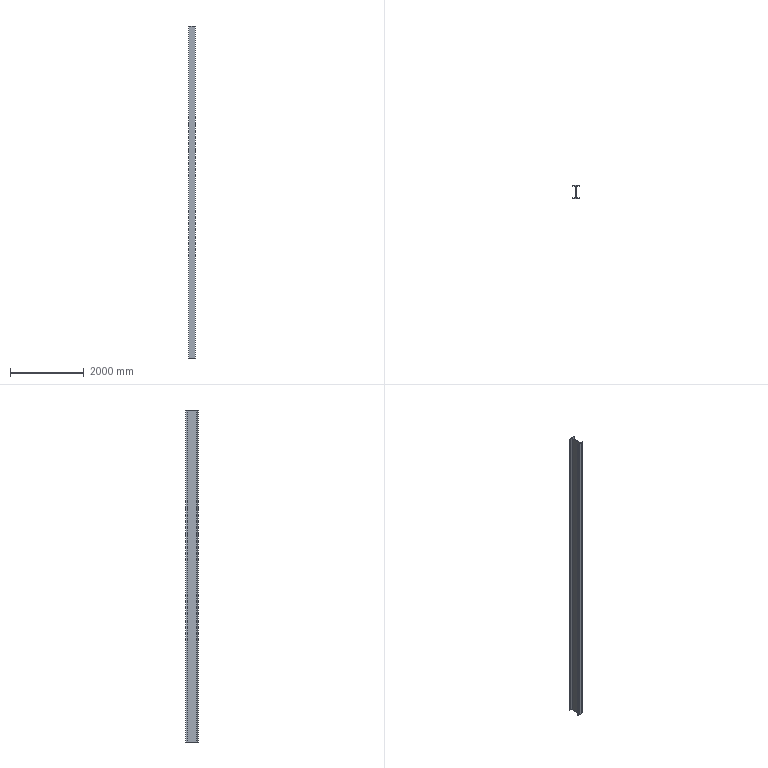Part | STEP file | 1 solid | 18 faces | box 175 x 350 x 9000 mm | volume 85369066 mm3 | plane 14 | cylinder 4 | commonest cylinder face diameters 80 x4
STEP:
#1=CARTESIAN_POINT('',(0.,0.,0.));
#2=DIRECTION('',(0.,0.,1.));
#3=DIRECTION('',(1.,0.,0.));
#4=AXIS2_PLACEMENT_3D('',#1,#2,#3);
#5=CARTESIAN_POINT('',(2499.715,-4168.542,-4500.));
#6=VERTEX_POINT('',#5);
#7=CARTESIAN_POINT('',(2499.715,-4156.542,-4500.));
#8=VERTEX_POINT('',#7);
#9=CARTESIAN_POINT('',(2499.715,-4156.542,-4500.));
#10=DIRECTION('',(0.,1.,0.));
#11=VECTOR('',#10,1.);
#12=LINE('',#9,#11);
#13=CARTESIAN_POINT('',(2499.715,-4156.542,4500.));
#14=DIRECTION('',(-1.,0.,0.));
#15=DIRECTION('',(0.,0.,1.));
#16=AXIS2_PLACEMENT_3D('',#13,#14,#15);
#17=PLANE('',#16);
#18=CARTESIAN_POINT('',(-9000.,0.));
#19=DIRECTION('',(0.,1.));
#20=VECTOR('',#19,1.);
#21=LINE('',#18,#20);
#22=(GEOMETRIC_REPRESENTATION_CONTEXT(2)PARAMETRIC_REPRESENTATION_CONTEXT()REPRESENTATION_CONTEXT('',''));
#23=DEFINITIONAL_REPRESENTATION('',(#21),#22);
#24=PCURVE('',#17,#23);
#25=CARTESIAN_POINT('',(2458.215,-4208.542,-4500.));
#26=DIRECTION('',(0.,0.,1.));
#27=DIRECTION('',(1.,0.,0.));
#28=AXIS2_PLACEMENT_3D('',#25,#26,#27);
#29=PLANE('',#28);
#30=CARTESIAN_POINT('',(41.5,52.));
#31=DIRECTION('',(0.,1.));
#32=VECTOR('',#31,1.);
#33=LINE('',#30,#32);
#34=(GEOMETRIC_REPRESENTATION_CONTEXT(2)PARAMETRIC_REPRESENTATION_CONTEXT()REPRESENTATION_CONTEXT('',''));
#35=DEFINITIONAL_REPRESENTATION('',(#33),#34);
#36=PCURVE('',#29,#35);
#37=SURFACE_CURVE('',#12,(#24,#36),.PCURVE_S1.);
#38=EDGE_CURVE('',#6,#8,#37,.T.);
#39=ORIENTED_EDGE('',*,*,#38,.T.);
#40=CARTESIAN_POINT('',(2499.715,-4156.542,4500.));
#41=VERTEX_POINT('',#40);
#42=CARTESIAN_POINT('',(2499.715,-4156.542,4500.));
#43=DIRECTION('',(0.,0.,-1.));
#44=VECTOR('',#43,1.);
#45=LINE('',#42,#44);
#46=CARTESIAN_POINT('',(0.,0.));
#47=DIRECTION('',(-1.,0.));
#48=VECTOR('',#47,1.);
#49=LINE('',#46,#48);
#50=(GEOMETRIC_REPRESENTATION_CONTEXT(2)PARAMETRIC_REPRESENTATION_CONTEXT()REPRESENTATION_CONTEXT('',''));
#51=DEFINITIONAL_REPRESENTATION('',(#49),#50);
#52=PCURVE('',#17,#51);
#53=CARTESIAN_POINT('',(2499.715,-4156.542,4500.));
#54=DIRECTION('',(0.,-1.,0.));
#55=DIRECTION('',(0.,0.,-1.));
#56=AXIS2_PLACEMENT_3D('',#53,#54,#55);
#57=PLANE('',#56);
#58=CARTESIAN_POINT('',(0.,0.));
#59=DIRECTION('',(1.,0.));
#60=VECTOR('',#59,1.);
#61=LINE('',#58,#60);
#62=(GEOMETRIC_REPRESENTATION_CONTEXT(2)PARAMETRIC_REPRESENTATION_CONTEXT()REPRESENTATION_CONTEXT('',''));
#63=DEFINITIONAL_REPRESENTATION('',(#61),#62);
#64=PCURVE('',#57,#63);
#65=SURFACE_CURVE('',#45,(#52,#64),.PCURVE_S1.);
#66=EDGE_CURVE('',#41,#8,#65,.T.);
#67=ORIENTED_EDGE('',*,*,#66,.F.);
#68=CARTESIAN_POINT('',(2499.715,-4168.542,4500.));
#69=VERTEX_POINT('',#68);
#70=CARTESIAN_POINT('',(2499.715,-4156.542,4500.));
#71=DIRECTION('',(0.,1.,0.));
#72=VECTOR('',#71,1.);
#73=LINE('',#70,#72);
#74=CARTESIAN_POINT('',(0.,0.));
#75=DIRECTION('',(0.,1.));
#76=VECTOR('',#75,1.);
#77=LINE('',#74,#76);
#78=(GEOMETRIC_REPRESENTATION_CONTEXT(2)PARAMETRIC_REPRESENTATION_CONTEXT()REPRESENTATION_CONTEXT('',''));
#79=DEFINITIONAL_REPRESENTATION('',(#77),#78);
#80=PCURVE('',#17,#79);
#81=CARTESIAN_POINT('',(2458.215,-4208.542,4500.));
#82=DIRECTION('',(0.,0.,1.));
#83=DIRECTION('',(1.,0.,0.));
#84=AXIS2_PLACEMENT_3D('',#81,#82,#83);
#85=PLANE('',#84);
#86=CARTESIAN_POINT('',(41.5,52.));
#87=DIRECTION('',(0.,1.));
#88=VECTOR('',#87,1.);
#89=LINE('',#86,#88);
#90=(GEOMETRIC_REPRESENTATION_CONTEXT(2)PARAMETRIC_REPRESENTATION_CONTEXT()REPRESENTATION_CONTEXT('',''));
#91=DEFINITIONAL_REPRESENTATION('',(#89),#90);
#92=PCURVE('',#85,#91);
#93=SURFACE_CURVE('',#73,(#80,#92),.PCURVE_S1.);
#94=EDGE_CURVE('',#69,#41,#93,.T.);
#95=ORIENTED_EDGE('',*,*,#94,.F.);
#96=CARTESIAN_POINT('',(2499.715,-4168.542,4500.));
#97=DIRECTION('',(0.,0.,-1.));
#98=VECTOR('',#97,1.);
#99=LINE('',#96,#98);
#100=CARTESIAN_POINT('',(0.,-12.));
#101=DIRECTION('',(-1.,0.));
#102=VECTOR('',#101,1.);
#103=LINE('',#100,#102);
#104=(GEOMETRIC_REPRESENTATION_CONTEXT(2)PARAMETRIC_REPRESENTATION_CONTEXT()REPRESENTATION_CONTEXT('',''));
#105=DEFINITIONAL_REPRESENTATION('',(#103),#104);
#106=PCURVE('',#17,#105);
#107=CARTESIAN_POINT('',(2499.715,-4168.542,4500.));
#108=DIRECTION('',(0.,1.,0.));
#109=DIRECTION('',(0.,0.,1.));
#110=AXIS2_PLACEMENT_3D('',#107,#108,#109);
#111=PLANE('',#110);
#112=CARTESIAN_POINT('',(0.,0.));
#113=DIRECTION('',(-1.,0.));
#114=VECTOR('',#113,1.);
#115=LINE('',#112,#114);
#116=(GEOMETRIC_REPRESENTATION_CONTEXT(2)PARAMETRIC_REPRESENTATION_CONTEXT()REPRESENTATION_CONTEXT('',''));
#117=DEFINITIONAL_REPRESENTATION('',(#115),#116);
#118=PCURVE('',#111,#117);
#119=SURFACE_CURVE('',#99,(#106,#118),.PCURVE_S1.);
#120=EDGE_CURVE('',#69,#6,#119,.T.);
#121=ORIENTED_EDGE('',*,*,#120,.T.);
#122=EDGE_LOOP('',(#39,#67,#95,#121));
#123=FACE_BOUND('',#122,.T.);
#124=ADVANCED_FACE('',(#123),#17,.F.);
#125=CARTESIAN_POINT('',(2324.715,-4156.542,-4500.));
#126=VERTEX_POINT('',#125);
#127=CARTESIAN_POINT('',(2499.715,-4156.542,-4500.));
#128=DIRECTION('',(-1.,0.,0.));
#129=VECTOR('',#128,1.);
#130=LINE('',#127,#129);
#131=CARTESIAN_POINT('',(9000.,0.));
#132=DIRECTION('',(0.,-1.));
#133=VECTOR('',#132,1.);
#134=LINE('',#131,#133);
#135=(GEOMETRIC_REPRESENTATION_CONTEXT(2)PARAMETRIC_REPRESENTATION_CONTEXT()REPRESENTATION_CONTEXT('',''));
#136=DEFINITIONAL_REPRESENTATION('',(#134),#135);
#137=PCURVE('',#57,#136);
#138=CARTESIAN_POINT('',(41.5,52.));
#139=DIRECTION('',(-1.,0.));
#140=VECTOR('',#139,1.);
#141=LINE('',#138,#140);
#142=(GEOMETRIC_REPRESENTATION_CONTEXT(2)PARAMETRIC_REPRESENTATION_CONTEXT()REPRESENTATION_CONTEXT('',''));
#143=DEFINITIONAL_REPRESENTATION('',(#141),#142);
#144=PCURVE('',#29,#143);
#145=SURFACE_CURVE('',#130,(#137,#144),.PCURVE_S1.);
#146=EDGE_CURVE('',#8,#126,#145,.T.);
#147=ORIENTED_EDGE('',*,*,#146,.T.);
#148=CARTESIAN_POINT('',(2324.715,-4156.542,4500.));
#149=VERTEX_POINT('',#148);
#150=CARTESIAN_POINT('',(2324.715,-4156.542,4500.));
#151=DIRECTION('',(0.,0.,-1.));
#152=VECTOR('',#151,1.);
#153=LINE('',#150,#152);
#154=CARTESIAN_POINT('',(0.,-175.));
#155=DIRECTION('',(1.,0.));
#156=VECTOR('',#155,1.);
#157=LINE('',#154,#156);
#158=(GEOMETRIC_REPRESENTATION_CONTEXT(2)PARAMETRIC_REPRESENTATION_CONTEXT()REPRESENTATION_CONTEXT('',''));
#159=DEFINITIONAL_REPRESENTATION('',(#157),#158);
#160=PCURVE('',#57,#159);
#161=CARTESIAN_POINT('',(2324.715,-4156.542,4500.));
#162=DIRECTION('',(1.,0.,0.));
#163=DIRECTION('',(0.,0.,-1.));
#164=AXIS2_PLACEMENT_3D('',#161,#162,#163);
#165=PLANE('',#164);
#166=CARTESIAN_POINT('',(0.,0.));
#167=DIRECTION('',(1.,0.));
#168=VECTOR('',#167,1.);
#169=LINE('',#166,#168);
#170=(GEOMETRIC_REPRESENTATION_CONTEXT(2)PARAMETRIC_REPRESENTATION_CONTEXT()REPRESENTATION_CONTEXT('',''));
#171=DEFINITIONAL_REPRESENTATION('',(#169),#170);
#172=PCURVE('',#165,#171);
#173=SURFACE_CURVE('',#153,(#160,#172),.PCURVE_S1.);
#174=EDGE_CURVE('',#149,#126,#173,.T.);
#175=ORIENTED_EDGE('',*,*,#174,.F.);
#176=CARTESIAN_POINT('',(2499.715,-4156.542,4500.));
#177=DIRECTION('',(-1.,0.,0.));
#178=VECTOR('',#177,1.);
#179=LINE('',#176,#178);
#180=CARTESIAN_POINT('',(0.,0.));
#181=DIRECTION('',(0.,-1.));
#182=VECTOR('',#181,1.);
#183=LINE('',#180,#182);
#184=(GEOMETRIC_REPRESENTATION_CONTEXT(2)PARAMETRIC_REPRESENTATION_CONTEXT()REPRESENTATION_CONTEXT('',''));
#185=DEFINITIONAL_REPRESENTATION('',(#183),#184);
#186=PCURVE('',#57,#185);
#187=CARTESIAN_POINT('',(41.5,52.));
#188=DIRECTION('',(-1.,0.));
#189=VECTOR('',#188,1.);
#190=LINE('',#187,#189);
#191=(GEOMETRIC_REPRESENTATION_CONTEXT(2)PARAMETRIC_REPRESENTATION_CONTEXT()REPRESENTATION_CONTEXT('',''));
#192=DEFINITIONAL_REPRESENTATION('',(#190),#191);
#193=PCURVE('',#85,#192);
#194=SURFACE_CURVE('',#179,(#186,#193),.PCURVE_S1.);
#195=EDGE_CURVE('',#41,#149,#194,.T.);
#196=ORIENTED_EDGE('',*,*,#195,.F.);
#197=ORIENTED_EDGE('',*,*,#66,.T.);
#198=EDGE_LOOP('',(#147,#175,#196,#197));
#199=FACE_BOUND('',#198,.T.);
#200=ADVANCED_FACE('',(#199),#57,.F.);
#201=CARTESIAN_POINT('',(2324.715,-4168.542,-4500.));
#202=VERTEX_POINT('',#201);
#203=CARTESIAN_POINT('',(2324.715,-4156.542,-4500.));
#204=DIRECTION('',(0.,-1.,0.));
#205=VECTOR('',#204,1.);
#206=LINE('',#203,#205);
#207=CARTESIAN_POINT('',(9000.,0.));
#208=DIRECTION('',(0.,-1.));
#209=VECTOR('',#208,1.);
#210=LINE('',#207,#209);
#211=(GEOMETRIC_REPRESENTATION_CONTEXT(2)PARAMETRIC_REPRESENTATION_CONTEXT()REPRESENTATION_CONTEXT('',''));
#212=DEFINITIONAL_REPRESENTATION('',(#210),#211);
#213=PCURVE('',#165,#212);
#214=CARTESIAN_POINT('',(-133.5,52.));
#215=DIRECTION('',(0.,-1.));
#216=VECTOR('',#215,1.);
#217=LINE('',#214,#216);
#218=(GEOMETRIC_REPRESENTATION_CONTEXT(2)PARAMETRIC_REPRESENTATION_CONTEXT()REPRESENTATION_CONTEXT('',''));
#219=DEFINITIONAL_REPRESENTATION('',(#217),#218);
#220=PCURVE('',#29,#219);
#221=SURFACE_CURVE('',#206,(#213,#220),.PCURVE_S1.);
#222=EDGE_CURVE('',#126,#202,#221,.T.);
#223=ORIENTED_EDGE('',*,*,#222,.T.);
#224=CARTESIAN_POINT('',(2324.715,-4168.542,4500.));
#225=VERTEX_POINT('',#224);
#226=CARTESIAN_POINT('',(2324.715,-4168.542,4500.));
#227=DIRECTION('',(0.,0.,-1.));
#228=VECTOR('',#227,1.);
#229=LINE('',#226,#228);
#230=CARTESIAN_POINT('',(0.,-12.));
#231=DIRECTION('',(1.,0.));
#232=VECTOR('',#231,1.);
#233=LINE('',#230,#232);
#234=(GEOMETRIC_REPRESENTATION_CONTEXT(2)PARAMETRIC_REPRESENTATION_CONTEXT()REPRESENTATION_CONTEXT('',''));
#235=DEFINITIONAL_REPRESENTATION('',(#233),#234);
#236=PCURVE('',#165,#235);
#237=CARTESIAN_POINT('',(2366.215,-4168.542,4500.));
#238=DIRECTION('',(0.,1.,0.));
#239=DIRECTION('',(0.,0.,1.));
#240=AXIS2_PLACEMENT_3D('',#237,#238,#239);
#241=PLANE('',#240);
#242=CARTESIAN_POINT('',(0.,-41.5));
#243=DIRECTION('',(-1.,0.));
#244=VECTOR('',#243,1.);
#245=LINE('',#242,#244);
#246=(GEOMETRIC_REPRESENTATION_CONTEXT(2)PARAMETRIC_REPRESENTATION_CONTEXT()REPRESENTATION_CONTEXT('',''));
#247=DEFINITIONAL_REPRESENTATION('',(#245),#246);
#248=PCURVE('',#241,#247);
#249=SURFACE_CURVE('',#229,(#236,#248),.PCURVE_S1.);
#250=EDGE_CURVE('',#225,#202,#249,.T.);
#251=ORIENTED_EDGE('',*,*,#250,.F.);
#252=CARTESIAN_POINT('',(2324.715,-4156.542,4500.));
#253=DIRECTION('',(0.,-1.,0.));
#254=VECTOR('',#253,1.);
#255=LINE('',#252,#254);
#256=CARTESIAN_POINT('',(0.,0.));
#257=DIRECTION('',(0.,-1.));
#258=VECTOR('',#257,1.);
#259=LINE('',#256,#258);
#260=(GEOMETRIC_REPRESENTATION_CONTEXT(2)PARAMETRIC_REPRESENTATION_CONTEXT()REPRESENTATION_CONTEXT('',''));
#261=DEFINITIONAL_REPRESENTATION('',(#259),#260);
#262=PCURVE('',#165,#261);
#263=CARTESIAN_POINT('',(-133.5,52.));
#264=DIRECTION('',(0.,-1.));
#265=VECTOR('',#264,1.);
#266=LINE('',#263,#265);
#267=(GEOMETRIC_REPRESENTATION_CONTEXT(2)PARAMETRIC_REPRESENTATION_CONTEXT()REPRESENTATION_CONTEXT('',''));
#268=DEFINITIONAL_REPRESENTATION('',(#266),#267);
#269=PCURVE('',#85,#268);
#270=SURFACE_CURVE('',#255,(#262,#269),.PCURVE_S1.);
#271=EDGE_CURVE('',#149,#225,#270,.T.);
#272=ORIENTED_EDGE('',*,*,#271,.F.);
#273=ORIENTED_EDGE('',*,*,#174,.T.);
#274=EDGE_LOOP('',(#223,#251,#272,#273));
#275=FACE_BOUND('',#274,.T.);
#276=ADVANCED_FACE('',(#275),#165,.F.);
#277=CARTESIAN_POINT('',(2366.215,-4168.542,-4500.));
#278=VERTEX_POINT('',#277);
#279=CARTESIAN_POINT('',(2366.215,-4168.542,-4500.));
#280=DIRECTION('',(1.,0.,0.));
#281=VECTOR('',#280,1.);
#282=LINE('',#279,#281);
#283=CARTESIAN_POINT('',(-9000.,0.));
#284=DIRECTION('',(0.,1.));
#285=VECTOR('',#284,1.);
#286=LINE('',#283,#285);
#287=(GEOMETRIC_REPRESENTATION_CONTEXT(2)PARAMETRIC_REPRESENTATION_CONTEXT()REPRESENTATION_CONTEXT('',''));
#288=DEFINITIONAL_REPRESENTATION('',(#286),#287);
#289=PCURVE('',#241,#288);
#290=CARTESIAN_POINT('',(-92.,40.));
#291=DIRECTION('',(1.,0.));
#292=VECTOR('',#291,1.);
#293=LINE('',#290,#292);
#294=(GEOMETRIC_REPRESENTATION_CONTEXT(2)PARAMETRIC_REPRESENTATION_CONTEXT()REPRESENTATION_CONTEXT('',''));
#295=DEFINITIONAL_REPRESENTATION('',(#293),#294);
#296=PCURVE('',#29,#295);
#297=SURFACE_CURVE('',#282,(#289,#296),.PCURVE_S1.);
#298=EDGE_CURVE('',#202,#278,#297,.T.);
#299=ORIENTED_EDGE('',*,*,#298,.T.);
#300=CARTESIAN_POINT('',(2366.215,-4168.542,4500.));
#301=VERTEX_POINT('',#300);
#302=CARTESIAN_POINT('',(2366.215,-4168.542,4500.));
#303=DIRECTION('',(0.,0.,-1.));
#304=VECTOR('',#303,1.);
#305=LINE('',#302,#304);
#306=CARTESIAN_POINT('',(0.,0.));
#307=DIRECTION('',(-1.,0.));
#308=VECTOR('',#307,1.);
#309=LINE('',#306,#308);
#310=(GEOMETRIC_REPRESENTATION_CONTEXT(2)PARAMETRIC_REPRESENTATION_CONTEXT()REPRESENTATION_CONTEXT('',''));
#311=DEFINITIONAL_REPRESENTATION('',(#309),#310);
#312=PCURVE('',#241,#311);
#313=CARTESIAN_POINT('',(2366.215,-4208.542,4500.));
#314=DIRECTION('',(0.,0.,-1.));
#315=DIRECTION('',(-1.,0.,0.));
#316=AXIS2_PLACEMENT_3D('',#313,#314,#315);
#317=CYLINDRICAL_SURFACE('',#316,40.);
#318=CARTESIAN_POINT('',(1.571,0.));
#319=DIRECTION('',(0.,1.));
#320=VECTOR('',#319,1.);
#321=LINE('',#318,#320);
#322=(GEOMETRIC_REPRESENTATION_CONTEXT(2)PARAMETRIC_REPRESENTATION_CONTEXT()REPRESENTATION_CONTEXT('',''));
#323=DEFINITIONAL_REPRESENTATION('',(#321),#322);
#324=PCURVE('',#317,#323);
#325=SURFACE_CURVE('',#305,(#312,#324),.PCURVE_S1.);
#326=EDGE_CURVE('',#301,#278,#325,.T.);
#327=ORIENTED_EDGE('',*,*,#326,.F.);
#328=CARTESIAN_POINT('',(2366.215,-4168.542,4500.));
#329=DIRECTION('',(1.,0.,0.));
#330=VECTOR('',#329,1.);
#331=LINE('',#328,#330);
#332=CARTESIAN_POINT('',(0.,0.));
#333=DIRECTION('',(0.,1.));
#334=VECTOR('',#333,1.);
#335=LINE('',#332,#334);
#336=(GEOMETRIC_REPRESENTATION_CONTEXT(2)PARAMETRIC_REPRESENTATION_CONTEXT()REPRESENTATION_CONTEXT('',''));
#337=DEFINITIONAL_REPRESENTATION('',(#335),#336);
#338=PCURVE('',#241,#337);
#339=CARTESIAN_POINT('',(-92.,40.));
#340=DIRECTION('',(1.,0.));
#341=VECTOR('',#340,1.);
#342=LINE('',#339,#341);
#343=(GEOMETRIC_REPRESENTATION_CONTEXT(2)PARAMETRIC_REPRESENTATION_CONTEXT()REPRESENTATION_CONTEXT('',''));
#344=DEFINITIONAL_REPRESENTATION('',(#342),#343);
#345=PCURVE('',#85,#344);
#346=SURFACE_CURVE('',#331,(#338,#345),.PCURVE_S1.);
#347=EDGE_CURVE('',#225,#301,#346,.T.);
#348=ORIENTED_EDGE('',*,*,#347,.F.);
#349=ORIENTED_EDGE('',*,*,#250,.T.);
#350=EDGE_LOOP('',(#299,#327,#348,#349));
#351=FACE_BOUND('',#350,.T.);
#352=ADVANCED_FACE('',(#351),#241,.F.);
#353=ORIENTED_EDGE('',*,*,#326,.F.);
#354=CARTESIAN_POINT('',(2406.215,-4208.542,4500.));
#355=VERTEX_POINT('',#354);
#356=CARTESIAN_POINT('',(2366.215,-4208.542,4500.));
#357=DIRECTION('',(0.,0.,-1.));
#358=DIRECTION('',(1.,0.,0.));
#359=AXIS2_PLACEMENT_3D('',#356,#357,#358);
#360=CIRCLE('',#359,40.);
#361=CARTESIAN_POINT('',(-3.142,0.));
#362=DIRECTION('',(1.,0.));
#363=VECTOR('',#362,1.);
#364=LINE('',#361,#363);
#365=(GEOMETRIC_REPRESENTATION_CONTEXT(2)PARAMETRIC_REPRESENTATION_CONTEXT()REPRESENTATION_CONTEXT('',''));
#366=DEFINITIONAL_REPRESENTATION('',(#364),#365);
#367=PCURVE('',#317,#366);
#368=CARTESIAN_POINT('',(-52.,0.));
#369=CARTESIAN_POINT('',(-52.,-69.282));
#370=CARTESIAN_POINT('',(-112.,-34.641));
#371=CARTESIAN_POINT('',(-172.,0.));
#372=CARTESIAN_POINT('',(-112.,34.641));
#373=CARTESIAN_POINT('',(-52.,69.282));
#374=CARTESIAN_POINT('',(-52.,0.));
#375=(BOUNDED_CURVE()B_SPLINE_CURVE(2,(#368,#369,#370,#371,#372,#373,#374),.UNSPECIFIED.,.T.,.F.)B_SPLINE_CURVE_WITH_KNOTS((1,2,2,2,2,1),(-2.094,0.,2.094,4.189,6.283,8.378),.UNSPECIFIED.)CURVE()GEOMETRIC_REPRESENTATION_ITEM()RATIONAL_B_SPLINE_CURVE((1.,0.5,1.,0.5,1.,0.5,1.))REPRESENTATION_ITEM(''));
#376=(GEOMETRIC_REPRESENTATION_CONTEXT(2)PARAMETRIC_REPRESENTATION_CONTEXT()REPRESENTATION_CONTEXT('',''));
#377=DEFINITIONAL_REPRESENTATION('',(#375),#376);
#378=PCURVE('',#85,#377);
#379=SURFACE_CURVE('',#360,(#367,#378),.PCURVE_S1.);
#380=EDGE_CURVE('',#301,#355,#379,.T.);
#381=ORIENTED_EDGE('',*,*,#380,.T.);
#382=CARTESIAN_POINT('',(2406.215,-4208.542,-4500.));
#383=VERTEX_POINT('',#382);
#384=CARTESIAN_POINT('',(2406.215,-4208.542,4500.));
#385=DIRECTION('',(0.,0.,-1.));
#386=VECTOR('',#385,1.);
#387=LINE('',#384,#386);
#388=CARTESIAN_POINT('',(3.142,0.));
#389=DIRECTION('',(0.,1.));
#390=VECTOR('',#389,1.);
#391=LINE('',#388,#390);
#392=(GEOMETRIC_REPRESENTATION_CONTEXT(2)PARAMETRIC_REPRESENTATION_CONTEXT()REPRESENTATION_CONTEXT('',''));
#393=DEFINITIONAL_REPRESENTATION('',(#391),#392);
#394=PCURVE('',#317,#393);
#395=CARTESIAN_POINT('',(2406.215,-4208.542,4500.));
#396=DIRECTION('',(1.,0.,0.));
#397=DIRECTION('',(0.,0.,-1.));
#398=AXIS2_PLACEMENT_3D('',#395,#396,#397);
#399=PLANE('',#398);
#400=CARTESIAN_POINT('',(0.,0.));
#401=DIRECTION('',(1.,0.));
#402=VECTOR('',#401,1.);
#403=LINE('',#400,#402);
#404=(GEOMETRIC_REPRESENTATION_CONTEXT(2)PARAMETRIC_REPRESENTATION_CONTEXT()REPRESENTATION_CONTEXT('',''));
#405=DEFINITIONAL_REPRESENTATION('',(#403),#404);
#406=PCURVE('',#399,#405);
#407=SURFACE_CURVE('',#387,(#394,#406),.PCURVE_S1.);
#408=EDGE_CURVE('',#355,#383,#407,.T.);
#409=ORIENTED_EDGE('',*,*,#408,.T.);
#410=CARTESIAN_POINT('',(2366.215,-4208.542,-4500.));
#411=DIRECTION('',(0.,0.,-1.));
#412=DIRECTION('',(1.,0.,0.));
#413=AXIS2_PLACEMENT_3D('',#410,#411,#412);
#414=CIRCLE('',#413,40.);
#415=CARTESIAN_POINT('',(-3.142,9000.));
#416=DIRECTION('',(1.,0.));
#417=VECTOR('',#416,1.);
#418=LINE('',#415,#417);
#419=(GEOMETRIC_REPRESENTATION_CONTEXT(2)PARAMETRIC_REPRESENTATION_CONTEXT()REPRESENTATION_CONTEXT('',''));
#420=DEFINITIONAL_REPRESENTATION('',(#418),#419);
#421=PCURVE('',#317,#420);
#422=CARTESIAN_POINT('',(-52.,0.));
#423=CARTESIAN_POINT('',(-52.,-69.282));
#424=CARTESIAN_POINT('',(-112.,-34.641));
#425=CARTESIAN_POINT('',(-172.,0.));
#426=CARTESIAN_POINT('',(-112.,34.641));
#427=CARTESIAN_POINT('',(-52.,69.282));
#428=CARTESIAN_POINT('',(-52.,0.));
#429=(BOUNDED_CURVE()B_SPLINE_CURVE(2,(#422,#423,#424,#425,#426,#427,#428),.UNSPECIFIED.,.T.,.F.)B_SPLINE_CURVE_WITH_KNOTS((1,2,2,2,2,1),(-2.094,0.,2.094,4.189,6.283,8.378),.UNSPECIFIED.)CURVE()GEOMETRIC_REPRESENTATION_ITEM()RATIONAL_B_SPLINE_CURVE((1.,0.5,1.,0.5,1.,0.5,1.))REPRESENTATION_ITEM(''));
#430=(GEOMETRIC_REPRESENTATION_CONTEXT(2)PARAMETRIC_REPRESENTATION_CONTEXT()REPRESENTATION_CONTEXT('',''));
#431=DEFINITIONAL_REPRESENTATION('',(#429),#430);
#432=PCURVE('',#29,#431);
#433=SURFACE_CURVE('',#414,(#421,#432),.PCURVE_S1.);
#434=EDGE_CURVE('',#278,#383,#433,.T.);
#435=ORIENTED_EDGE('',*,*,#434,.F.);
#436=EDGE_LOOP('',(#353,#381,#409,#435));
#437=FACE_BOUND('',#436,.F.);
#438=ADVANCED_FACE('',(#437),#317,.F.);
#439=CARTESIAN_POINT('',(2406.215,-4454.542,-4500.));
#440=VERTEX_POINT('',#439);
#441=CARTESIAN_POINT('',(2406.215,-4208.542,-4500.));
#442=DIRECTION('',(0.,-1.,0.));
#443=VECTOR('',#442,1.);
#444=LINE('',#441,#443);
#445=CARTESIAN_POINT('',(9000.,0.));
#446=DIRECTION('',(0.,-1.));
#447=VECTOR('',#446,1.);
#448=LINE('',#445,#447);
#449=(GEOMETRIC_REPRESENTATION_CONTEXT(2)PARAMETRIC_REPRESENTATION_CONTEXT()REPRESENTATION_CONTEXT('',''));
#450=DEFINITIONAL_REPRESENTATION('',(#448),#449);
#451=PCURVE('',#399,#450);
#452=CARTESIAN_POINT('',(-52.,0.));
#453=DIRECTION('',(0.,-1.));
#454=VECTOR('',#453,1.);
#455=LINE('',#452,#454);
#456=(GEOMETRIC_REPRESENTATION_CONTEXT(2)PARAMETRIC_REPRESENTATION_CONTEXT()REPRESENTATION_CONTEXT('',''));
#457=DEFINITIONAL_REPRESENTATION('',(#455),#456);
#458=PCURVE('',#29,#457);
#459=SURFACE_CURVE('',#444,(#451,#458),.PCURVE_S1.);
#460=EDGE_CURVE('',#383,#440,#459,.T.);
#461=ORIENTED_EDGE('',*,*,#460,.T.);
#462=CARTESIAN_POINT('',(2406.215,-4454.542,4500.));
#463=VERTEX_POINT('',#462);
#464=CARTESIAN_POINT('',(2406.215,-4454.542,4500.));
#465=DIRECTION('',(0.,0.,-1.));
#466=VECTOR('',#465,1.);
#467=LINE('',#464,#466);
#468=CARTESIAN_POINT('',(0.,-246.));
#469=DIRECTION('',(1.,0.));
#470=VECTOR('',#469,1.);
#471=LINE('',#468,#470);
#472=(GEOMETRIC_REPRESENTATION_CONTEXT(2)PARAMETRIC_REPRESENTATION_CONTEXT()REPRESENTATION_CONTEXT('',''));
#473=DEFINITIONAL_REPRESENTATION('',(#471),#472);
#474=PCURVE('',#399,#473);
#475=CARTESIAN_POINT('',(2366.215,-4454.542,4500.));
#476=DIRECTION('',(0.,0.,-1.));
#477=DIRECTION('',(-1.,0.,0.));
#478=AXIS2_PLACEMENT_3D('',#475,#476,#477);
#479=CYLINDRICAL_SURFACE('',#478,40.);
#480=CARTESIAN_POINT('',(3.142,0.));
#481=DIRECTION('',(0.,1.));
#482=VECTOR('',#481,1.);
#483=LINE('',#480,#482);
#484=(GEOMETRIC_REPRESENTATION_CONTEXT(2)PARAMETRIC_REPRESENTATION_CONTEXT()REPRESENTATION_CONTEXT('',''));
#485=DEFINITIONAL_REPRESENTATION('',(#483),#484);
#486=PCURVE('',#479,#485);
#487=SURFACE_CURVE('',#467,(#474,#486),.PCURVE_S1.);
#488=EDGE_CURVE('',#463,#440,#487,.T.);
#489=ORIENTED_EDGE('',*,*,#488,.F.);
#490=CARTESIAN_POINT('',(2406.215,-4208.542,4500.));
#491=DIRECTION('',(0.,-1.,0.));
#492=VECTOR('',#491,1.);
#493=LINE('',#490,#492);
#494=CARTESIAN_POINT('',(0.,0.));
#495=DIRECTION('',(0.,-1.));
#496=VECTOR('',#495,1.);
#497=LINE('',#494,#496);
#498=(GEOMETRIC_REPRESENTATION_CONTEXT(2)PARAMETRIC_REPRESENTATION_CONTEXT()REPRESENTATION_CONTEXT('',''));
#499=DEFINITIONAL_REPRESENTATION('',(#497),#498);
#500=PCURVE('',#399,#499);
#501=CARTESIAN_POINT('',(-52.,0.));
#502=DIRECTION('',(0.,-1.));
#503=VECTOR('',#502,1.);
#504=LINE('',#501,#503);
#505=(GEOMETRIC_REPRESENTATION_CONTEXT(2)PARAMETRIC_REPRESENTATION_CONTEXT()REPRESENTATION_CONTEXT('',''));
#506=DEFINITIONAL_REPRESENTATION('',(#504),#505);
#507=PCURVE('',#85,#506);
#508=SURFACE_CURVE('',#493,(#500,#507),.PCURVE_S1.);
#509=EDGE_CURVE('',#355,#463,#508,.T.);
#510=ORIENTED_EDGE('',*,*,#509,.F.);
#511=ORIENTED_EDGE('',*,*,#408,.T.);
#512=EDGE_LOOP('',(#461,#489,#510,#511));
#513=FACE_BOUND('',#512,.T.);
#514=ADVANCED_FACE('',(#513),#399,.F.);
#515=ORIENTED_EDGE('',*,*,#488,.F.);
#516=CARTESIAN_POINT('',(2366.215,-4494.542,4500.));
#517=VERTEX_POINT('',#516);
#518=CARTESIAN_POINT('',(2366.215,-4454.542,4500.));
#519=DIRECTION('',(0.,0.,-1.));
#520=DIRECTION('',(1.,0.,0.));
#521=AXIS2_PLACEMENT_3D('',#518,#519,#520);
#522=CIRCLE('',#521,40.);
#523=CARTESIAN_POINT('',(3.142,0.));
#524=DIRECTION('',(1.,0.));
#525=VECTOR('',#524,1.);
#526=LINE('',#523,#525);
#527=(GEOMETRIC_REPRESENTATION_CONTEXT(2)PARAMETRIC_REPRESENTATION_CONTEXT()REPRESENTATION_CONTEXT('',''));
#528=DEFINITIONAL_REPRESENTATION('',(#526),#527);
#529=PCURVE('',#479,#528);
#530=CARTESIAN_POINT('',(-52.,-246.));
#531=CARTESIAN_POINT('',(-52.,-315.282));
#532=CARTESIAN_POINT('',(-112.,-280.641));
#533=CARTESIAN_POINT('',(-172.,-246.));
#534=CARTESIAN_POINT('',(-112.,-211.359));
#535=CARTESIAN_POINT('',(-52.,-176.718));
#536=CARTESIAN_POINT('',(-52.,-246.));
#537=(BOUNDED_CURVE()B_SPLINE_CURVE(2,(#530,#531,#532,#533,#534,#535,#536),.UNSPECIFIED.,.T.,.F.)B_SPLINE_CURVE_WITH_KNOTS((1,2,2,2,2,1),(-2.094,0.,2.094,4.189,6.283,8.378),.UNSPECIFIED.)CURVE()GEOMETRIC_REPRESENTATION_ITEM()RATIONAL_B_SPLINE_CURVE((1.,0.5,1.,0.5,1.,0.5,1.))REPRESENTATION_ITEM(''));
#538=(GEOMETRIC_REPRESENTATION_CONTEXT(2)PARAMETRIC_REPRESENTATION_CONTEXT()REPRESENTATION_CONTEXT('',''));
#539=DEFINITIONAL_REPRESENTATION('',(#537),#538);
#540=PCURVE('',#85,#539);
#541=SURFACE_CURVE('',#522,(#529,#540),.PCURVE_S1.);
#542=EDGE_CURVE('',#463,#517,#541,.T.);
#543=ORIENTED_EDGE('',*,*,#542,.T.);
#544=CARTESIAN_POINT('',(2366.215,-4494.542,-4500.));
#545=VERTEX_POINT('',#544);
#546=CARTESIAN_POINT('',(2366.215,-4494.542,4500.));
#547=DIRECTION('',(0.,0.,-1.));
#548=VECTOR('',#547,1.);
#549=LINE('',#546,#548);
#550=CARTESIAN_POINT('',(4.712,0.));
#551=DIRECTION('',(0.,1.));
#552=VECTOR('',#551,1.);
#553=LINE('',#550,#552);
#554=(GEOMETRIC_REPRESENTATION_CONTEXT(2)PARAMETRIC_REPRESENTATION_CONTEXT()REPRESENTATION_CONTEXT('',''));
#555=DEFINITIONAL_REPRESENTATION('',(#553),#554);
#556=PCURVE('',#479,#555);
#557=CARTESIAN_POINT('',(2366.215,-4494.542,4500.));
#558=DIRECTION('',(0.,-1.,0.));
#559=DIRECTION('',(0.,0.,-1.));
#560=AXIS2_PLACEMENT_3D('',#557,#558,#559);
#561=PLANE('',#560);
#562=CARTESIAN_POINT('',(0.,0.));
#563=DIRECTION('',(1.,0.));
#564=VECTOR('',#563,1.);
#565=LINE('',#562,#564);
#566=(GEOMETRIC_REPRESENTATION_CONTEXT(2)PARAMETRIC_REPRESENTATION_CONTEXT()REPRESENTATION_CONTEXT('',''));
#567=DEFINITIONAL_REPRESENTATION('',(#565),#566);
#568=PCURVE('',#561,#567);
#569=SURFACE_CURVE('',#549,(#556,#568),.PCURVE_S1.);
#570=EDGE_CURVE('',#517,#545,#569,.T.);
#571=ORIENTED_EDGE('',*,*,#570,.T.);
#572=CARTESIAN_POINT('',(2366.215,-4454.542,-4500.));
#573=DIRECTION('',(0.,0.,-1.));
#574=DIRECTION('',(1.,0.,0.));
#575=AXIS2_PLACEMENT_3D('',#572,#573,#574);
#576=CIRCLE('',#575,40.);
#577=CARTESIAN_POINT('',(3.142,9000.));
#578=DIRECTION('',(1.,0.));
#579=VECTOR('',#578,1.);
#580=LINE('',#577,#579);
#581=(GEOMETRIC_REPRESENTATION_CONTEXT(2)PARAMETRIC_REPRESENTATION_CONTEXT()REPRESENTATION_CONTEXT('',''));
#582=DEFINITIONAL_REPRESENTATION('',(#580),#581);
#583=PCURVE('',#479,#582);
#584=CARTESIAN_POINT('',(-52.,-246.));
#585=CARTESIAN_POINT('',(-52.,-315.282));
#586=CARTESIAN_POINT('',(-112.,-280.641));
#587=CARTESIAN_POINT('',(-172.,-246.));
#588=CARTESIAN_POINT('',(-112.,-211.359));
#589=CARTESIAN_POINT('',(-52.,-176.718));
#590=CARTESIAN_POINT('',(-52.,-246.));
#591=(BOUNDED_CURVE()B_SPLINE_CURVE(2,(#584,#585,#586,#587,#588,#589,#590),.UNSPECIFIED.,.T.,.F.)B_SPLINE_CURVE_WITH_KNOTS((1,2,2,2,2,1),(-2.094,0.,2.094,4.189,6.283,8.378),.UNSPECIFIED.)CURVE()GEOMETRIC_REPRESENTATION_ITEM()RATIONAL_B_SPLINE_CURVE((1.,0.5,1.,0.5,1.,0.5,1.))REPRESENTATION_ITEM(''));
#592=(GEOMETRIC_REPRESENTATION_CONTEXT(2)PARAMETRIC_REPRESENTATION_CONTEXT()REPRESENTATION_CONTEXT('',''));
#593=DEFINITIONAL_REPRESENTATION('',(#591),#592);
#594=PCURVE('',#29,#593);
#595=SURFACE_CURVE('',#576,(#583,#594),.PCURVE_S1.);
#596=EDGE_CURVE('',#440,#545,#595,.T.);
#597=ORIENTED_EDGE('',*,*,#596,.F.);
#598=EDGE_LOOP('',(#515,#543,#571,#597));
#599=FACE_BOUND('',#598,.F.);
#600=ADVANCED_FACE('',(#599),#479,.F.);
#601=CARTESIAN_POINT('',(2324.715,-4494.542,-4500.));
#602=VERTEX_POINT('',#601);
#603=CARTESIAN_POINT('',(2366.215,-4494.542,-4500.));
#604=DIRECTION('',(-1.,0.,0.));
#605=VECTOR('',#604,1.);
#606=LINE('',#603,#605);
#607=CARTESIAN_POINT('',(9000.,0.));
#608=DIRECTION('',(0.,-1.));
#609=VECTOR('',#608,1.);
#610=LINE('',#607,#609);
#611=(GEOMETRIC_REPRESENTATION_CONTEXT(2)PARAMETRIC_REPRESENTATION_CONTEXT()REPRESENTATION_CONTEXT('',''));
#612=DEFINITIONAL_REPRESENTATION('',(#610),#611);
#613=PCURVE('',#561,#612);
#614=CARTESIAN_POINT('',(-92.,-286.));
#615=DIRECTION('',(-1.,0.));
#616=VECTOR('',#615,1.);
#617=LINE('',#614,#616);
#618=(GEOMETRIC_REPRESENTATION_CONTEXT(2)PARAMETRIC_REPRESENTATION_CONTEXT()REPRESENTATION_CONTEXT('',''));
#619=DEFINITIONAL_REPRESENTATION('',(#617),#618);
#620=PCURVE('',#29,#619);
#621=SURFACE_CURVE('',#606,(#613,#620),.PCURVE_S1.);
#622=EDGE_CURVE('',#545,#602,#621,.T.);
#623=ORIENTED_EDGE('',*,*,#622,.T.);
#624=CARTESIAN_POINT('',(2324.715,-4494.542,4500.));
#625=VERTEX_POINT('',#624);
#626=CARTESIAN_POINT('',(2324.715,-4494.542,4500.));
#627=DIRECTION('',(0.,0.,-1.));
#628=VECTOR('',#627,1.);
#629=LINE('',#626,#628);
#630=CARTESIAN_POINT('',(0.,-41.5));
#631=DIRECTION('',(1.,0.));
#632=VECTOR('',#631,1.);
#633=LINE('',#630,#632);
#634=(GEOMETRIC_REPRESENTATION_CONTEXT(2)PARAMETRIC_REPRESENTATION_CONTEXT()REPRESENTATION_CONTEXT('',''));
#635=DEFINITIONAL_REPRESENTATION('',(#633),#634);
#636=PCURVE('',#561,#635);
#637=CARTESIAN_POINT('',(2324.715,-4506.542,4500.));
#638=DIRECTION('',(1.,0.,0.));
#639=DIRECTION('',(0.,0.,-1.));
#640=AXIS2_PLACEMENT_3D('',#637,#638,#639);
#641=PLANE('',#640);
#642=CARTESIAN_POINT('',(0.,12.));
#643=DIRECTION('',(1.,0.));
#644=VECTOR('',#643,1.);
#645=LINE('',#642,#644);
#646=(GEOMETRIC_REPRESENTATION_CONTEXT(2)PARAMETRIC_REPRESENTATION_CONTEXT()REPRESENTATION_CONTEXT('',''));
#647=DEFINITIONAL_REPRESENTATION('',(#645),#646);
#648=PCURVE('',#641,#647);
#649=SURFACE_CURVE('',#629,(#636,#648),.PCURVE_S1.);
#650=EDGE_CURVE('',#625,#602,#649,.T.);
#651=ORIENTED_EDGE('',*,*,#650,.F.);
#652=CARTESIAN_POINT('',(2366.215,-4494.542,4500.));
#653=DIRECTION('',(-1.,0.,0.));
#654=VECTOR('',#653,1.);
#655=LINE('',#652,#654);
#656=CARTESIAN_POINT('',(0.,0.));
#657=DIRECTION('',(0.,-1.));
#658=VECTOR('',#657,1.);
#659=LINE('',#656,#658);
#660=(GEOMETRIC_REPRESENTATION_CONTEXT(2)PARAMETRIC_REPRESENTATION_CONTEXT()REPRESENTATION_CONTEXT('',''));
#661=DEFINITIONAL_REPRESENTATION('',(#659),#660);
#662=PCURVE('',#561,#661);
#663=CARTESIAN_POINT('',(-92.,-286.));
#664=DIRECTION('',(-1.,0.));
#665=VECTOR('',#664,1.);
#666=LINE('',#663,#665);
#667=(GEOMETRIC_REPRESENTATION_CONTEXT(2)PARAMETRIC_REPRESENTATION_CONTEXT()REPRESENTATION_CONTEXT('',''));
#668=DEFINITIONAL_REPRESENTATION('',(#666),#667);
#669=PCURVE('',#85,#668);
#670=SURFACE_CURVE('',#655,(#662,#669),.PCURVE_S1.);
#671=EDGE_CURVE('',#517,#625,#670,.T.);
#672=ORIENTED_EDGE('',*,*,#671,.F.);
#673=ORIENTED_EDGE('',*,*,#570,.T.);
#674=EDGE_LOOP('',(#623,#651,#672,#673));
#675=FACE_BOUND('',#674,.T.);
#676=ADVANCED_FACE('',(#675),#561,.F.);
#677=CARTESIAN_POINT('',(2324.715,-4506.542,-4500.));
#678=VERTEX_POINT('',#677);
#679=CARTESIAN_POINT('',(2324.715,-4506.542,-4500.));
#680=DIRECTION('',(0.,-1.,0.));
#681=VECTOR('',#680,1.);
#682=LINE('',#679,#681);
#683=CARTESIAN_POINT('',(9000.,0.));
#684=DIRECTION('',(0.,-1.));
#685=VECTOR('',#684,1.);
#686=LINE('',#683,#685);
#687=(GEOMETRIC_REPRESENTATION_CONTEXT(2)PARAMETRIC_REPRESENTATION_CONTEXT()REPRESENTATION_CONTEXT('',''));
#688=DEFINITIONAL_REPRESENTATION('',(#686),#687);
#689=PCURVE('',#641,#688);
#690=CARTESIAN_POINT('',(-133.5,-298.));
#691=DIRECTION('',(0.,-1.));
#692=VECTOR('',#691,1.);
#693=LINE('',#690,#692);
#694=(GEOMETRIC_REPRESENTATION_CONTEXT(2)PARAMETRIC_REPRESENTATION_CONTEXT()REPRESENTATION_CONTEXT('',''));
#695=DEFINITIONAL_REPRESENTATION('',(#693),#694);
#696=PCURVE('',#29,#695);
#697=SURFACE_CURVE('',#682,(#689,#696),.PCURVE_S1.);
#698=EDGE_CURVE('',#602,#678,#697,.T.);
#699=ORIENTED_EDGE('',*,*,#698,.T.);
#700=CARTESIAN_POINT('',(2324.715,-4506.542,4500.));
#701=VERTEX_POINT('',#700);
#702=CARTESIAN_POINT('',(2324.715,-4506.542,4500.));
#703=DIRECTION('',(0.,0.,-1.));
#704=VECTOR('',#703,1.);
#705=LINE('',#702,#704);
#706=CARTESIAN_POINT('',(0.,0.));
#707=DIRECTION('',(1.,0.));
#708=VECTOR('',#707,1.);
#709=LINE('',#706,#708);
#710=(GEOMETRIC_REPRESENTATION_CONTEXT(2)PARAMETRIC_REPRESENTATION_CONTEXT()REPRESENTATION_CONTEXT('',''));
#711=DEFINITIONAL_REPRESENTATION('',(#709),#710);
#712=PCURVE('',#641,#711);
#713=CARTESIAN_POINT('',(2499.715,-4506.542,4500.));
#714=DIRECTION('',(0.,1.,0.));
#715=DIRECTION('',(-1.,0.,0.));
#716=AXIS2_PLACEMENT_3D('',#713,#714,#715);
#717=PLANE('',#716);
#718=CARTESIAN_POINT('',(175.,0.));
#719=DIRECTION('',(0.,-1.));
#720=VECTOR('',#719,1.);
#721=LINE('',#718,#720);
#722=(GEOMETRIC_REPRESENTATION_CONTEXT(2)PARAMETRIC_REPRESENTATION_CONTEXT()REPRESENTATION_CONTEXT('',''));
#723=DEFINITIONAL_REPRESENTATION('',(#721),#722);
#724=PCURVE('',#717,#723);
#725=SURFACE_CURVE('',#705,(#712,#724),.PCURVE_S1.);
#726=EDGE_CURVE('',#701,#678,#725,.T.);
#727=ORIENTED_EDGE('',*,*,#726,.F.);
#728=CARTESIAN_POINT('',(2324.715,-4506.542,4500.));
#729=DIRECTION('',(0.,-1.,0.));
#730=VECTOR('',#729,1.);
#731=LINE('',#728,#730);
#732=CARTESIAN_POINT('',(0.,0.));
#733=DIRECTION('',(0.,-1.));
#734=VECTOR('',#733,1.);
#735=LINE('',#732,#734);
#736=(GEOMETRIC_REPRESENTATION_CONTEXT(2)PARAMETRIC_REPRESENTATION_CONTEXT()REPRESENTATION_CONTEXT('',''));
#737=DEFINITIONAL_REPRESENTATION('',(#735),#736);
#738=PCURVE('',#641,#737);
#739=CARTESIAN_POINT('',(-133.5,-298.));
#740=DIRECTION('',(0.,-1.));
#741=VECTOR('',#740,1.);
#742=LINE('',#739,#741);
#743=(GEOMETRIC_REPRESENTATION_CONTEXT(2)PARAMETRIC_REPRESENTATION_CONTEXT()REPRESENTATION_CONTEXT('',''));
#744=DEFINITIONAL_REPRESENTATION('',(#742),#743);
#745=PCURVE('',#85,#744);
#746=SURFACE_CURVE('',#731,(#738,#745),.PCURVE_S1.);
#747=EDGE_CURVE('',#625,#701,#746,.T.);
#748=ORIENTED_EDGE('',*,*,#747,.F.);
#749=ORIENTED_EDGE('',*,*,#650,.T.);
#750=EDGE_LOOP('',(#699,#727,#748,#749));
#751=FACE_BOUND('',#750,.T.);
#752=ADVANCED_FACE('',(#751),#641,.F.);
#753=CARTESIAN_POINT('',(2499.715,-4506.542,-4500.));
#754=VERTEX_POINT('',#753);
#755=CARTESIAN_POINT('',(2499.715,-4506.542,-4500.));
#756=DIRECTION('',(1.,0.,0.));
#757=VECTOR('',#756,1.);
#758=LINE('',#755,#757);
#759=CARTESIAN_POINT('',(0.,-9000.));
#760=DIRECTION('',(-1.,0.));
#761=VECTOR('',#760,1.);
#762=LINE('',#759,#761);
#763=(GEOMETRIC_REPRESENTATION_CONTEXT(2)PARAMETRIC_REPRESENTATION_CONTEXT()REPRESENTATION_CONTEXT('',''));
#764=DEFINITIONAL_REPRESENTATION('',(#762),#763);
#765=PCURVE('',#717,#764);
#766=CARTESIAN_POINT('',(41.5,-298.));
#767=DIRECTION('',(1.,0.));
#768=VECTOR('',#767,1.);
#769=LINE('',#766,#768);
#770=(GEOMETRIC_REPRESENTATION_CONTEXT(2)PARAMETRIC_REPRESENTATION_CONTEXT()REPRESENTATION_CONTEXT('',''));
#771=DEFINITIONAL_REPRESENTATION('',(#769),#770);
#772=PCURVE('',#29,#771);
#773=SURFACE_CURVE('',#758,(#765,#772),.PCURVE_S1.);
#774=EDGE_CURVE('',#678,#754,#773,.T.);
#775=ORIENTED_EDGE('',*,*,#774,.T.);
#776=CARTESIAN_POINT('',(2499.715,-4506.542,4500.));
#777=VERTEX_POINT('',#776);
#778=CARTESIAN_POINT('',(2499.715,-4506.542,4500.));
#779=DIRECTION('',(0.,0.,-1.));
#780=VECTOR('',#779,1.);
#781=LINE('',#778,#780);
#782=CARTESIAN_POINT('',(0.,0.));
#783=DIRECTION('',(0.,-1.));
#784=VECTOR('',#783,1.);
#785=LINE('',#782,#784);
#786=(GEOMETRIC_REPRESENTATION_CONTEXT(2)PARAMETRIC_REPRESENTATION_CONTEXT()REPRESENTATION_CONTEXT('',''));
#787=DEFINITIONAL_REPRESENTATION('',(#785),#786);
#788=PCURVE('',#717,#787);
#789=CARTESIAN_POINT('',(2499.715,-4506.542,4500.));
#790=DIRECTION('',(-1.,0.,0.));
#791=DIRECTION('',(0.,0.,1.));
#792=AXIS2_PLACEMENT_3D('',#789,#790,#791);
#793=PLANE('',#792);
#794=CARTESIAN_POINT('',(0.,0.));
#795=DIRECTION('',(-1.,0.));
#796=VECTOR('',#795,1.);
#797=LINE('',#794,#796);
#798=(GEOMETRIC_REPRESENTATION_CONTEXT(2)PARAMETRIC_REPRESENTATION_CONTEXT()REPRESENTATION_CONTEXT('',''));
#799=DEFINITIONAL_REPRESENTATION('',(#797),#798);
#800=PCURVE('',#793,#799);
#801=SURFACE_CURVE('',#781,(#788,#800),.PCURVE_S1.);
#802=EDGE_CURVE('',#777,#754,#801,.T.);
#803=ORIENTED_EDGE('',*,*,#802,.F.);
#804=CARTESIAN_POINT('',(2499.715,-4506.542,4500.));
#805=DIRECTION('',(1.,0.,0.));
#806=VECTOR('',#805,1.);
#807=LINE('',#804,#806);
#808=CARTESIAN_POINT('',(0.,0.));
#809=DIRECTION('',(-1.,0.));
#810=VECTOR('',#809,1.);
#811=LINE('',#808,#810);
#812=(GEOMETRIC_REPRESENTATION_CONTEXT(2)PARAMETRIC_REPRESENTATION_CONTEXT()REPRESENTATION_CONTEXT('',''));
#813=DEFINITIONAL_REPRESENTATION('',(#811),#812);
#814=PCURVE('',#717,#813);
#815=CARTESIAN_POINT('',(41.5,-298.));
#816=DIRECTION('',(1.,0.));
#817=VECTOR('',#816,1.);
#818=LINE('',#815,#817);
#819=(GEOMETRIC_REPRESENTATION_CONTEXT(2)PARAMETRIC_REPRESENTATION_CONTEXT()REPRESENTATION_CONTEXT('',''));
#820=DEFINITIONAL_REPRESENTATION('',(#818),#819);
#821=PCURVE('',#85,#820);
#822=SURFACE_CURVE('',#807,(#814,#821),.PCURVE_S1.);
#823=EDGE_CURVE('',#701,#777,#822,.T.);
#824=ORIENTED_EDGE('',*,*,#823,.F.);
#825=ORIENTED_EDGE('',*,*,#726,.T.);
#826=EDGE_LOOP('',(#775,#803,#824,#825));
#827=FACE_BOUND('',#826,.T.);
#828=ADVANCED_FACE('',(#827),#717,.F.);
#829=CARTESIAN_POINT('',(2499.715,-4494.542,-4500.));
#830=VERTEX_POINT('',#829);
#831=CARTESIAN_POINT('',(2499.715,-4506.542,-4500.));
#832=DIRECTION('',(0.,1.,0.));
#833=VECTOR('',#832,1.);
#834=LINE('',#831,#833);
#835=CARTESIAN_POINT('',(-9000.,0.));
#836=DIRECTION('',(0.,1.));
#837=VECTOR('',#836,1.);
#838=LINE('',#835,#837);
#839=(GEOMETRIC_REPRESENTATION_CONTEXT(2)PARAMETRIC_REPRESENTATION_CONTEXT()REPRESENTATION_CONTEXT('',''));
#840=DEFINITIONAL_REPRESENTATION('',(#838),#839);
#841=PCURVE('',#793,#840);
#842=CARTESIAN_POINT('',(41.5,-298.));
#843=DIRECTION('',(0.,1.));
#844=VECTOR('',#843,1.);
#845=LINE('',#842,#844);
#846=(GEOMETRIC_REPRESENTATION_CONTEXT(2)PARAMETRIC_REPRESENTATION_CONTEXT()REPRESENTATION_CONTEXT('',''));
#847=DEFINITIONAL_REPRESENTATION('',(#845),#846);
#848=PCURVE('',#29,#847);
#849=SURFACE_CURVE('',#834,(#841,#848),.PCURVE_S1.);
#850=EDGE_CURVE('',#754,#830,#849,.T.);
#851=ORIENTED_EDGE('',*,*,#850,.T.);
#852=CARTESIAN_POINT('',(2499.715,-4494.542,4500.));
#853=VERTEX_POINT('',#852);
#854=CARTESIAN_POINT('',(2499.715,-4494.542,4500.));
#855=DIRECTION('',(0.,0.,-1.));
#856=VECTOR('',#855,1.);
#857=LINE('',#854,#856);
#858=CARTESIAN_POINT('',(0.,12.));
#859=DIRECTION('',(-1.,0.));
#860=VECTOR('',#859,1.);
#861=LINE('',#858,#860);
#862=(GEOMETRIC_REPRESENTATION_CONTEXT(2)PARAMETRIC_REPRESENTATION_CONTEXT()REPRESENTATION_CONTEXT('',''));
#863=DEFINITIONAL_REPRESENTATION('',(#861),#862);
#864=PCURVE('',#793,#863);
#865=CARTESIAN_POINT('',(2499.715,-4494.542,4500.));
#866=DIRECTION('',(0.,-1.,0.));
#867=DIRECTION('',(0.,0.,-1.));
#868=AXIS2_PLACEMENT_3D('',#865,#866,#867);
#869=PLANE('',#868);
#870=CARTESIAN_POINT('',(0.,0.));
#871=DIRECTION('',(1.,0.));
#872=VECTOR('',#871,1.);
#873=LINE('',#870,#872);
#874=(GEOMETRIC_REPRESENTATION_CONTEXT(2)PARAMETRIC_REPRESENTATION_CONTEXT()REPRESENTATION_CONTEXT('',''));
#875=DEFINITIONAL_REPRESENTATION('',(#873),#874);
#876=PCURVE('',#869,#875);
#877=SURFACE_CURVE('',#857,(#864,#876),.PCURVE_S1.);
#878=EDGE_CURVE('',#853,#830,#877,.T.);
#879=ORIENTED_EDGE('',*,*,#878,.F.);
#880=CARTESIAN_POINT('',(2499.715,-4506.542,4500.));
#881=DIRECTION('',(0.,1.,0.));
#882=VECTOR('',#881,1.);
#883=LINE('',#880,#882);
#884=CARTESIAN_POINT('',(0.,0.));
#885=DIRECTION('',(0.,1.));
#886=VECTOR('',#885,1.);
#887=LINE('',#884,#886);
#888=(GEOMETRIC_REPRESENTATION_CONTEXT(2)PARAMETRIC_REPRESENTATION_CONTEXT()REPRESENTATION_CONTEXT('',''));
#889=DEFINITIONAL_REPRESENTATION('',(#887),#888);
#890=PCURVE('',#793,#889);
#891=CARTESIAN_POINT('',(41.5,-298.));
#892=DIRECTION('',(0.,1.));
#893=VECTOR('',#892,1.);
#894=LINE('',#891,#893);
#895=(GEOMETRIC_REPRESENTATION_CONTEXT(2)PARAMETRIC_REPRESENTATION_CONTEXT()REPRESENTATION_CONTEXT('',''));
#896=DEFINITIONAL_REPRESENTATION('',(#894),#895);
#897=PCURVE('',#85,#896);
#898=SURFACE_CURVE('',#883,(#890,#897),.PCURVE_S1.);
#899=EDGE_CURVE('',#777,#853,#898,.T.);
#900=ORIENTED_EDGE('',*,*,#899,.F.);
#901=ORIENTED_EDGE('',*,*,#802,.T.);
#902=EDGE_LOOP('',(#851,#879,#900,#901));
#903=FACE_BOUND('',#902,.T.);
#904=ADVANCED_FACE('',(#903),#793,.F.);
#905=CARTESIAN_POINT('',(2458.215,-4494.542,-4500.));
#906=VERTEX_POINT('',#905);
#907=CARTESIAN_POINT('',(2499.715,-4494.542,-4500.));
#908=DIRECTION('',(-1.,0.,0.));
#909=VECTOR('',#908,1.);
#910=LINE('',#907,#909);
#911=CARTESIAN_POINT('',(9000.,0.));
#912=DIRECTION('',(0.,-1.));
#913=VECTOR('',#912,1.);
#914=LINE('',#911,#913);
#915=(GEOMETRIC_REPRESENTATION_CONTEXT(2)PARAMETRIC_REPRESENTATION_CONTEXT()REPRESENTATION_CONTEXT('',''));
#916=DEFINITIONAL_REPRESENTATION('',(#914),#915);
#917=PCURVE('',#869,#916);
#918=CARTESIAN_POINT('',(41.5,-286.));
#919=DIRECTION('',(-1.,0.));
#920=VECTOR('',#919,1.);
#921=LINE('',#918,#920);
#922=(GEOMETRIC_REPRESENTATION_CONTEXT(2)PARAMETRIC_REPRESENTATION_CONTEXT()REPRESENTATION_CONTEXT('',''));
#923=DEFINITIONAL_REPRESENTATION('',(#921),#922);
#924=PCURVE('',#29,#923);
#925=SURFACE_CURVE('',#910,(#917,#924),.PCURVE_S1.);
#926=EDGE_CURVE('',#830,#906,#925,.T.);
#927=ORIENTED_EDGE('',*,*,#926,.T.);
#928=CARTESIAN_POINT('',(2458.215,-4494.542,4500.));
#929=VERTEX_POINT('',#928);
#930=CARTESIAN_POINT('',(2458.215,-4494.542,4500.));
#931=DIRECTION('',(0.,0.,-1.));
#932=VECTOR('',#931,1.);
#933=LINE('',#930,#932);
#934=CARTESIAN_POINT('',(0.,-41.5));
#935=DIRECTION('',(1.,0.));
#936=VECTOR('',#935,1.);
#937=LINE('',#934,#936);
#938=(GEOMETRIC_REPRESENTATION_CONTEXT(2)PARAMETRIC_REPRESENTATION_CONTEXT()REPRESENTATION_CONTEXT('',''));
#939=DEFINITIONAL_REPRESENTATION('',(#937),#938);
#940=PCURVE('',#869,#939);
#941=CARTESIAN_POINT('',(2458.215,-4454.542,4500.));
#942=DIRECTION('',(0.,0.,-1.));
#943=DIRECTION('',(-1.,0.,0.));
#944=AXIS2_PLACEMENT_3D('',#941,#942,#943);
#945=CYLINDRICAL_SURFACE('',#944,40.);
#946=CARTESIAN_POINT('',(4.712,0.));
#947=DIRECTION('',(0.,1.));
#948=VECTOR('',#947,1.);
#949=LINE('',#946,#948);
#950=(GEOMETRIC_REPRESENTATION_CONTEXT(2)PARAMETRIC_REPRESENTATION_CONTEXT()REPRESENTATION_CONTEXT('',''));
#951=DEFINITIONAL_REPRESENTATION('',(#949),#950);
#952=PCURVE('',#945,#951);
#953=SURFACE_CURVE('',#933,(#940,#952),.PCURVE_S1.);
#954=EDGE_CURVE('',#929,#906,#953,.T.);
#955=ORIENTED_EDGE('',*,*,#954,.F.);
#956=CARTESIAN_POINT('',(2499.715,-4494.542,4500.));
#957=DIRECTION('',(-1.,0.,0.));
#958=VECTOR('',#957,1.);
#959=LINE('',#956,#958);
#960=CARTESIAN_POINT('',(0.,0.));
#961=DIRECTION('',(0.,-1.));
#962=VECTOR('',#961,1.);
#963=LINE('',#960,#962);
#964=(GEOMETRIC_REPRESENTATION_CONTEXT(2)PARAMETRIC_REPRESENTATION_CONTEXT()REPRESENTATION_CONTEXT('',''));
#965=DEFINITIONAL_REPRESENTATION('',(#963),#964);
#966=PCURVE('',#869,#965);
#967=CARTESIAN_POINT('',(41.5,-286.));
#968=DIRECTION('',(-1.,0.));
#969=VECTOR('',#968,1.);
#970=LINE('',#967,#969);
#971=(GEOMETRIC_REPRESENTATION_CONTEXT(2)PARAMETRIC_REPRESENTATION_CONTEXT()REPRESENTATION_CONTEXT('',''));
#972=DEFINITIONAL_REPRESENTATION('',(#970),#971);
#973=PCURVE('',#85,#972);
#974=SURFACE_CURVE('',#959,(#966,#973),.PCURVE_S1.);
#975=EDGE_CURVE('',#853,#929,#974,.T.);
#976=ORIENTED_EDGE('',*,*,#975,.F.);
#977=ORIENTED_EDGE('',*,*,#878,.T.);
#978=EDGE_LOOP('',(#927,#955,#976,#977));
#979=FACE_BOUND('',#978,.T.);
#980=ADVANCED_FACE('',(#979),#869,.F.);
#981=ORIENTED_EDGE('',*,*,#954,.F.);
#982=CARTESIAN_POINT('',(2418.215,-4454.542,4500.));
#983=VERTEX_POINT('',#982);
#984=CARTESIAN_POINT('',(2458.215,-4454.542,4500.));
#985=DIRECTION('',(0.,0.,-1.));
#986=DIRECTION('',(1.,0.,0.));
#987=AXIS2_PLACEMENT_3D('',#984,#985,#986);
#988=CIRCLE('',#987,40.);
#989=CARTESIAN_POINT('',(3.142,0.));
#990=DIRECTION('',(1.,0.));
#991=VECTOR('',#990,1.);
#992=LINE('',#989,#991);
#993=(GEOMETRIC_REPRESENTATION_CONTEXT(2)PARAMETRIC_REPRESENTATION_CONTEXT()REPRESENTATION_CONTEXT('',''));
#994=DEFINITIONAL_REPRESENTATION('',(#992),#993);
#995=PCURVE('',#945,#994);
#996=CARTESIAN_POINT('',(40.,-246.));
#997=CARTESIAN_POINT('',(40.,-315.282));
#998=CARTESIAN_POINT('',(-20.,-280.641));
#999=CARTESIAN_POINT('',(-80.,-246.));
#1000=CARTESIAN_POINT('',(-20.,-211.359));
#1001=CARTESIAN_POINT('',(40.,-176.718));
#1002=CARTESIAN_POINT('',(40.,-246.));
#1003=(BOUNDED_CURVE()B_SPLINE_CURVE(2,(#996,#997,#998,#999,#1000,#1001,#1002),.UNSPECIFIED.,.T.,.F.)B_SPLINE_CURVE_WITH_KNOTS((1,2,2,2,2,1),(-2.094,0.,2.094,4.189,6.283,8.378),.UNSPECIFIED.)CURVE()GEOMETRIC_REPRESENTATION_ITEM()RATIONAL_B_SPLINE_CURVE((1.,0.5,1.,0.5,1.,0.5,1.))REPRESENTATION_ITEM(''));
#1004=(GEOMETRIC_REPRESENTATION_CONTEXT(2)PARAMETRIC_REPRESENTATION_CONTEXT()REPRESENTATION_CONTEXT('',''));
#1005=DEFINITIONAL_REPRESENTATION('',(#1003),#1004);
#1006=PCURVE('',#85,#1005);
#1007=SURFACE_CURVE('',#988,(#995,#1006),.PCURVE_S1.);
#1008=EDGE_CURVE('',#929,#983,#1007,.T.);
#1009=ORIENTED_EDGE('',*,*,#1008,.T.);
#1010=CARTESIAN_POINT('',(2418.215,-4454.542,-4500.));
#1011=VERTEX_POINT('',#1010);
#1012=CARTESIAN_POINT('',(2418.215,-4454.542,4500.));
#1013=DIRECTION('',(0.,0.,-1.));
#1014=VECTOR('',#1013,1.);
#1015=LINE('',#1012,#1014);
#1016=CARTESIAN_POINT('',(6.283,0.));
#1017=DIRECTION('',(0.,1.));
#1018=VECTOR('',#1017,1.);
#1019=LINE('',#1016,#1018);
#1020=(GEOMETRIC_REPRESENTATION_CONTEXT(2)PARAMETRIC_REPRESENTATION_CONTEXT()REPRESENTATION_CONTEXT('',''));
#1021=DEFINITIONAL_REPRESENTATION('',(#1019),#1020);
#1022=PCURVE('',#945,#1021);
#1023=CARTESIAN_POINT('',(2418.215,-4208.542,4500.));
#1024=DIRECTION('',(-1.,0.,0.));
#1025=DIRECTION('',(0.,0.,1.));
#1026=AXIS2_PLACEMENT_3D('',#1023,#1024,#1025);
#1027=PLANE('',#1026);
#1028=CARTESIAN_POINT('',(0.,-246.));
#1029=DIRECTION('',(-1.,0.));
#1030=VECTOR('',#1029,1.);
#1031=LINE('',#1028,#1030);
#1032=(GEOMETRIC_REPRESENTATION_CONTEXT(2)PARAMETRIC_REPRESENTATION_CONTEXT()REPRESENTATION_CONTEXT('',''));
#1033=DEFINITIONAL_REPRESENTATION('',(#1031),#1032);
#1034=PCURVE('',#1027,#1033);
#1035=SURFACE_CURVE('',#1015,(#1022,#1034),.PCURVE_S1.);
#1036=EDGE_CURVE('',#983,#1011,#1035,.T.);
#1037=ORIENTED_EDGE('',*,*,#1036,.T.);
#1038=CARTESIAN_POINT('',(2458.215,-4454.542,-4500.));
#1039=DIRECTION('',(0.,0.,-1.));
#1040=DIRECTION('',(1.,0.,0.));
#1041=AXIS2_PLACEMENT_3D('',#1038,#1039,#1040);
#1042=CIRCLE('',#1041,40.);
#1043=CARTESIAN_POINT('',(3.142,9000.));
#1044=DIRECTION('',(1.,0.));
#1045=VECTOR('',#1044,1.);
#1046=LINE('',#1043,#1045);
#1047=(GEOMETRIC_REPRESENTATION_CONTEXT(2)PARAMETRIC_REPRESENTATION_CONTEXT()REPRESENTATION_CONTEXT('',''));
#1048=DEFINITIONAL_REPRESENTATION('',(#1046),#1047);
#1049=PCURVE('',#945,#1048);
#1050=CARTESIAN_POINT('',(40.,-246.));
#1051=CARTESIAN_POINT('',(40.,-315.282));
#1052=CARTESIAN_POINT('',(-20.,-280.641));
#1053=CARTESIAN_POINT('',(-80.,-246.));
#1054=CARTESIAN_POINT('',(-20.,-211.359));
#1055=CARTESIAN_POINT('',(40.,-176.718));
#1056=CARTESIAN_POINT('',(40.,-246.));
#1057=(BOUNDED_CURVE()B_SPLINE_CURVE(2,(#1050,#1051,#1052,#1053,#1054,#1055,#1056),.UNSPECIFIED.,.T.,.F.)B_SPLINE_CURVE_WITH_KNOTS((1,2,2,2,2,1),(-2.094,0.,2.094,4.189,6.283,8.378),.UNSPECIFIED.)CURVE()GEOMETRIC_REPRESENTATION_ITEM()RATIONAL_B_SPLINE_CURVE((1.,0.5,1.,0.5,1.,0.5,1.))REPRESENTATION_ITEM(''));
#1058=(GEOMETRIC_REPRESENTATION_CONTEXT(2)PARAMETRIC_REPRESENTATION_CONTEXT()REPRESENTATION_CONTEXT('',''));
#1059=DEFINITIONAL_REPRESENTATION('',(#1057),#1058);
#1060=PCURVE('',#29,#1059);
#1061=SURFACE_CURVE('',#1042,(#1049,#1060),.PCURVE_S1.);
#1062=EDGE_CURVE('',#906,#1011,#1061,.T.);
#1063=ORIENTED_EDGE('',*,*,#1062,.F.);
#1064=EDGE_LOOP('',(#981,#1009,#1037,#1063));
#1065=FACE_BOUND('',#1064,.F.);
#1066=ADVANCED_FACE('',(#1065),#945,.F.);
#1067=CARTESIAN_POINT('',(2418.215,-4208.542,-4500.));
#1068=VERTEX_POINT('',#1067);
#1069=CARTESIAN_POINT('',(2418.215,-4208.542,-4500.));
#1070=DIRECTION('',(0.,1.,0.));
#1071=VECTOR('',#1070,1.);
#1072=LINE('',#1069,#1071);
#1073=CARTESIAN_POINT('',(-9000.,0.));
#1074=DIRECTION('',(0.,1.));
#1075=VECTOR('',#1074,1.);
#1076=LINE('',#1073,#1075);
#1077=(GEOMETRIC_REPRESENTATION_CONTEXT(2)PARAMETRIC_REPRESENTATION_CONTEXT()REPRESENTATION_CONTEXT('',''));
#1078=DEFINITIONAL_REPRESENTATION('',(#1076),#1077);
#1079=PCURVE('',#1027,#1078);
#1080=CARTESIAN_POINT('',(-40.,0.));
#1081=DIRECTION('',(0.,1.));
#1082=VECTOR('',#1081,1.);
#1083=LINE('',#1080,#1082);
#1084=(GEOMETRIC_REPRESENTATION_CONTEXT(2)PARAMETRIC_REPRESENTATION_CONTEXT()REPRESENTATION_CONTEXT('',''));
#1085=DEFINITIONAL_REPRESENTATION('',(#1083),#1084);
#1086=PCURVE('',#29,#1085);
#1087=SURFACE_CURVE('',#1072,(#1079,#1086),.PCURVE_S1.);
#1088=EDGE_CURVE('',#1011,#1068,#1087,.T.);
#1089=ORIENTED_EDGE('',*,*,#1088,.T.);
#1090=CARTESIAN_POINT('',(2418.215,-4208.542,4500.));
#1091=VERTEX_POINT('',#1090);
#1092=CARTESIAN_POINT('',(2418.215,-4208.542,4500.));
#1093=DIRECTION('',(0.,0.,-1.));
#1094=VECTOR('',#1093,1.);
#1095=LINE('',#1092,#1094);
#1096=CARTESIAN_POINT('',(0.,0.));
#1097=DIRECTION('',(-1.,0.));
#1098=VECTOR('',#1097,1.);
#1099=LINE('',#1096,#1098);
#1100=(GEOMETRIC_REPRESENTATION_CONTEXT(2)PARAMETRIC_REPRESENTATION_CONTEXT()REPRESENTATION_CONTEXT('',''));
#1101=DEFINITIONAL_REPRESENTATION('',(#1099),#1100);
#1102=PCURVE('',#1027,#1101);
#1103=CARTESIAN_POINT('',(2458.215,-4208.542,4500.));
#1104=DIRECTION('',(0.,0.,-1.));
#1105=DIRECTION('',(-1.,0.,0.));
#1106=AXIS2_PLACEMENT_3D('',#1103,#1104,#1105);
#1107=CYLINDRICAL_SURFACE('',#1106,40.);
#1108=CARTESIAN_POINT('',(0.,0.));
#1109=DIRECTION('',(0.,1.));
#1110=VECTOR('',#1109,1.);
#1111=LINE('',#1108,#1110);
#1112=(GEOMETRIC_REPRESENTATION_CONTEXT(2)PARAMETRIC_REPRESENTATION_CONTEXT()REPRESENTATION_CONTEXT('',''));
#1113=DEFINITIONAL_REPRESENTATION('',(#1111),#1112);
#1114=PCURVE('',#1107,#1113);
#1115=SURFACE_CURVE('',#1095,(#1102,#1114),.PCURVE_S1.);
#1116=EDGE_CURVE('',#1091,#1068,#1115,.T.);
#1117=ORIENTED_EDGE('',*,*,#1116,.F.);
#1118=CARTESIAN_POINT('',(2418.215,-4208.542,4500.));
#1119=DIRECTION('',(0.,1.,0.));
#1120=VECTOR('',#1119,1.);
#1121=LINE('',#1118,#1120);
#1122=CARTESIAN_POINT('',(0.,0.));
#1123=DIRECTION('',(0.,1.));
#1124=VECTOR('',#1123,1.);
#1125=LINE('',#1122,#1124);
#1126=(GEOMETRIC_REPRESENTATION_CONTEXT(2)PARAMETRIC_REPRESENTATION_CONTEXT()REPRESENTATION_CONTEXT('',''));
#1127=DEFINITIONAL_REPRESENTATION('',(#1125),#1126);
#1128=PCURVE('',#1027,#1127);
#1129=CARTESIAN_POINT('',(-40.,0.));
#1130=DIRECTION('',(0.,1.));
#1131=VECTOR('',#1130,1.);
#1132=LINE('',#1129,#1131);
#1133=(GEOMETRIC_REPRESENTATION_CONTEXT(2)PARAMETRIC_REPRESENTATION_CONTEXT()REPRESENTATION_CONTEXT('',''));
#1134=DEFINITIONAL_REPRESENTATION('',(#1132),#1133);
#1135=PCURVE('',#85,#1134);
#1136=SURFACE_CURVE('',#1121,(#1128,#1135),.PCURVE_S1.);
#1137=EDGE_CURVE('',#983,#1091,#1136,.T.);
#1138=ORIENTED_EDGE('',*,*,#1137,.F.);
#1139=ORIENTED_EDGE('',*,*,#1036,.T.);
#1140=EDGE_LOOP('',(#1089,#1117,#1138,#1139));
#1141=FACE_BOUND('',#1140,.T.);
#1142=ADVANCED_FACE('',(#1141),#1027,.F.);
#1143=ORIENTED_EDGE('',*,*,#1116,.F.);
#1144=CARTESIAN_POINT('',(2458.215,-4168.542,4500.));
#1145=VERTEX_POINT('',#1144);
#1146=CARTESIAN_POINT('',(2458.215,-4208.542,4500.));
#1147=DIRECTION('',(0.,0.,-1.));
#1148=DIRECTION('',(1.,0.,0.));
#1149=AXIS2_PLACEMENT_3D('',#1146,#1147,#1148);
#1150=CIRCLE('',#1149,40.);
#1151=CARTESIAN_POINT('',(-3.142,0.));
#1152=DIRECTION('',(1.,0.));
#1153=VECTOR('',#1152,1.);
#1154=LINE('',#1151,#1153);
#1155=(GEOMETRIC_REPRESENTATION_CONTEXT(2)PARAMETRIC_REPRESENTATION_CONTEXT()REPRESENTATION_CONTEXT('',''));
#1156=DEFINITIONAL_REPRESENTATION('',(#1154),#1155);
#1157=PCURVE('',#1107,#1156);
#1158=CARTESIAN_POINT('',(40.,0.));
#1159=CARTESIAN_POINT('',(40.,-69.282));
#1160=CARTESIAN_POINT('',(-20.,-34.641));
#1161=CARTESIAN_POINT('',(-80.,0.));
#1162=CARTESIAN_POINT('',(-20.,34.641));
#1163=CARTESIAN_POINT('',(40.,69.282));
#1164=CARTESIAN_POINT('',(40.,0.));
#1165=(BOUNDED_CURVE()B_SPLINE_CURVE(2,(#1158,#1159,#1160,#1161,#1162,#1163,#1164),.UNSPECIFIED.,.T.,.F.)B_SPLINE_CURVE_WITH_KNOTS((1,2,2,2,2,1),(-2.094,0.,2.094,4.189,6.283,8.378),.UNSPECIFIED.)CURVE()GEOMETRIC_REPRESENTATION_ITEM()RATIONAL_B_SPLINE_CURVE((1.,0.5,1.,0.5,1.,0.5,1.))REPRESENTATION_ITEM(''));
#1166=(GEOMETRIC_REPRESENTATION_CONTEXT(2)PARAMETRIC_REPRESENTATION_CONTEXT()REPRESENTATION_CONTEXT('',''));
#1167=DEFINITIONAL_REPRESENTATION('',(#1165),#1166);
#1168=PCURVE('',#85,#1167);
#1169=SURFACE_CURVE('',#1150,(#1157,#1168),.PCURVE_S1.);
#1170=EDGE_CURVE('',#1091,#1145,#1169,.T.);
#1171=ORIENTED_EDGE('',*,*,#1170,.T.);
#1172=CARTESIAN_POINT('',(2458.215,-4168.542,-4500.));
#1173=VERTEX_POINT('',#1172);
#1174=CARTESIAN_POINT('',(2458.215,-4168.542,4500.));
#1175=DIRECTION('',(0.,0.,-1.));
#1176=VECTOR('',#1175,1.);
#1177=LINE('',#1174,#1176);
#1178=CARTESIAN_POINT('',(1.571,0.));
#1179=DIRECTION('',(0.,1.));
#1180=VECTOR('',#1179,1.);
#1181=LINE('',#1178,#1180);
#1182=(GEOMETRIC_REPRESENTATION_CONTEXT(2)PARAMETRIC_REPRESENTATION_CONTEXT()REPRESENTATION_CONTEXT('',''));
#1183=DEFINITIONAL_REPRESENTATION('',(#1181),#1182);
#1184=PCURVE('',#1107,#1183);
#1185=CARTESIAN_POINT('',(0.,-41.5));
#1186=DIRECTION('',(-1.,0.));
#1187=VECTOR('',#1186,1.);
#1188=LINE('',#1185,#1187);
#1189=(GEOMETRIC_REPRESENTATION_CONTEXT(2)PARAMETRIC_REPRESENTATION_CONTEXT()REPRESENTATION_CONTEXT('',''));
#1190=DEFINITIONAL_REPRESENTATION('',(#1188),#1189);
#1191=PCURVE('',#111,#1190);
#1192=SURFACE_CURVE('',#1177,(#1184,#1191),.PCURVE_S1.);
#1193=EDGE_CURVE('',#1145,#1173,#1192,.T.);
#1194=ORIENTED_EDGE('',*,*,#1193,.T.);
#1195=CARTESIAN_POINT('',(2458.215,-4208.542,-4500.));
#1196=DIRECTION('',(0.,0.,-1.));
#1197=DIRECTION('',(1.,0.,0.));
#1198=AXIS2_PLACEMENT_3D('',#1195,#1196,#1197);
#1199=CIRCLE('',#1198,40.);
#1200=CARTESIAN_POINT('',(-3.142,9000.));
#1201=DIRECTION('',(1.,0.));
#1202=VECTOR('',#1201,1.);
#1203=LINE('',#1200,#1202);
#1204=(GEOMETRIC_REPRESENTATION_CONTEXT(2)PARAMETRIC_REPRESENTATION_CONTEXT()REPRESENTATION_CONTEXT('',''));
#1205=DEFINITIONAL_REPRESENTATION('',(#1203),#1204);
#1206=PCURVE('',#1107,#1205);
#1207=CARTESIAN_POINT('',(40.,0.));
#1208=CARTESIAN_POINT('',(40.,-69.282));
#1209=CARTESIAN_POINT('',(-20.,-34.641));
#1210=CARTESIAN_POINT('',(-80.,0.));
#1211=CARTESIAN_POINT('',(-20.,34.641));
#1212=CARTESIAN_POINT('',(40.,69.282));
#1213=CARTESIAN_POINT('',(40.,0.));
#1214=(BOUNDED_CURVE()B_SPLINE_CURVE(2,(#1207,#1208,#1209,#1210,#1211,#1212,#1213),.UNSPECIFIED.,.T.,.F.)B_SPLINE_CURVE_WITH_KNOTS((1,2,2,2,2,1),(-2.094,0.,2.094,4.189,6.283,8.378),.UNSPECIFIED.)CURVE()GEOMETRIC_REPRESENTATION_ITEM()RATIONAL_B_SPLINE_CURVE((1.,0.5,1.,0.5,1.,0.5,1.))REPRESENTATION_ITEM(''));
#1215=(GEOMETRIC_REPRESENTATION_CONTEXT(2)PARAMETRIC_REPRESENTATION_CONTEXT()REPRESENTATION_CONTEXT('',''));
#1216=DEFINITIONAL_REPRESENTATION('',(#1214),#1215);
#1217=PCURVE('',#29,#1216);
#1218=SURFACE_CURVE('',#1199,(#1206,#1217),.PCURVE_S1.);
#1219=EDGE_CURVE('',#1068,#1173,#1218,.T.);
#1220=ORIENTED_EDGE('',*,*,#1219,.F.);
#1221=EDGE_LOOP('',(#1143,#1171,#1194,#1220));
#1222=FACE_BOUND('',#1221,.F.);
#1223=ADVANCED_FACE('',(#1222),#1107,.F.);
#1224=CARTESIAN_POINT('',(2499.715,-4168.542,-4500.));
#1225=DIRECTION('',(1.,0.,0.));
#1226=VECTOR('',#1225,1.);
#1227=LINE('',#1224,#1226);
#1228=CARTESIAN_POINT('',(-9000.,0.));
#1229=DIRECTION('',(0.,1.));
#1230=VECTOR('',#1229,1.);
#1231=LINE('',#1228,#1230);
#1232=(GEOMETRIC_REPRESENTATION_CONTEXT(2)PARAMETRIC_REPRESENTATION_CONTEXT()REPRESENTATION_CONTEXT('',''));
#1233=DEFINITIONAL_REPRESENTATION('',(#1231),#1232);
#1234=PCURVE('',#111,#1233);
#1235=CARTESIAN_POINT('',(41.5,40.));
#1236=DIRECTION('',(1.,0.));
#1237=VECTOR('',#1236,1.);
#1238=LINE('',#1235,#1237);
#1239=(GEOMETRIC_REPRESENTATION_CONTEXT(2)PARAMETRIC_REPRESENTATION_CONTEXT()REPRESENTATION_CONTEXT('',''));
#1240=DEFINITIONAL_REPRESENTATION('',(#1238),#1239);
#1241=PCURVE('',#29,#1240);
#1242=SURFACE_CURVE('',#1227,(#1234,#1241),.PCURVE_S1.);
#1243=EDGE_CURVE('',#1173,#6,#1242,.T.);
#1244=ORIENTED_EDGE('',*,*,#1243,.T.);
#1245=ORIENTED_EDGE('',*,*,#120,.F.);
#1246=CARTESIAN_POINT('',(2499.715,-4168.542,4500.));
#1247=DIRECTION('',(1.,0.,0.));
#1248=VECTOR('',#1247,1.);
#1249=LINE('',#1246,#1248);
#1250=CARTESIAN_POINT('',(0.,0.));
#1251=DIRECTION('',(0.,1.));
#1252=VECTOR('',#1251,1.);
#1253=LINE('',#1250,#1252);
#1254=(GEOMETRIC_REPRESENTATION_CONTEXT(2)PARAMETRIC_REPRESENTATION_CONTEXT()REPRESENTATION_CONTEXT('',''));
#1255=DEFINITIONAL_REPRESENTATION('',(#1253),#1254);
#1256=PCURVE('',#111,#1255);
#1257=CARTESIAN_POINT('',(41.5,40.));
#1258=DIRECTION('',(1.,0.));
#1259=VECTOR('',#1258,1.);
#1260=LINE('',#1257,#1259);
#1261=(GEOMETRIC_REPRESENTATION_CONTEXT(2)PARAMETRIC_REPRESENTATION_CONTEXT()REPRESENTATION_CONTEXT('',''));
#1262=DEFINITIONAL_REPRESENTATION('',(#1260),#1261);
#1263=PCURVE('',#85,#1262);
#1264=SURFACE_CURVE('',#1249,(#1256,#1263),.PCURVE_S1.);
#1265=EDGE_CURVE('',#1145,#69,#1264,.T.);
#1266=ORIENTED_EDGE('',*,*,#1265,.F.);
#1267=ORIENTED_EDGE('',*,*,#1193,.T.);
#1268=EDGE_LOOP('',(#1244,#1245,#1266,#1267));
#1269=FACE_BOUND('',#1268,.T.);
#1270=ADVANCED_FACE('',(#1269),#111,.F.);
#1271=ORIENTED_EDGE('',*,*,#94,.T.);
#1272=ORIENTED_EDGE('',*,*,#195,.T.);
#1273=ORIENTED_EDGE('',*,*,#271,.T.);
#1274=ORIENTED_EDGE('',*,*,#347,.T.);
#1275=ORIENTED_EDGE('',*,*,#380,.T.);
#1276=ORIENTED_EDGE('',*,*,#509,.T.);
#1277=ORIENTED_EDGE('',*,*,#542,.T.);
#1278=ORIENTED_EDGE('',*,*,#671,.T.);
#1279=ORIENTED_EDGE('',*,*,#747,.T.);
#1280=ORIENTED_EDGE('',*,*,#823,.T.);
#1281=ORIENTED_EDGE('',*,*,#899,.T.);
#1282=ORIENTED_EDGE('',*,*,#975,.T.);
#1283=ORIENTED_EDGE('',*,*,#1008,.T.);
#1284=ORIENTED_EDGE('',*,*,#1137,.T.);
#1285=ORIENTED_EDGE('',*,*,#1170,.T.);
#1286=ORIENTED_EDGE('',*,*,#1265,.T.);
#1287=EDGE_LOOP('',(#1271,#1272,#1273,#1274,#1275,#1276,#1277,#1278,#1279,#1280,#1281,#1282,#1283,#1284,#1285,#1286));
#1288=FACE_BOUND('',#1287,.T.);
#1289=ADVANCED_FACE('',(#1288),#85,.T.);
#1290=ORIENTED_EDGE('',*,*,#38,.F.);
#1291=ORIENTED_EDGE('',*,*,#1243,.F.);
#1292=ORIENTED_EDGE('',*,*,#1219,.F.);
#1293=ORIENTED_EDGE('',*,*,#1088,.F.);
#1294=ORIENTED_EDGE('',*,*,#1062,.F.);
#1295=ORIENTED_EDGE('',*,*,#926,.F.);
#1296=ORIENTED_EDGE('',*,*,#850,.F.);
#1297=ORIENTED_EDGE('',*,*,#774,.F.);
#1298=ORIENTED_EDGE('',*,*,#698,.F.);
#1299=ORIENTED_EDGE('',*,*,#622,.F.);
#1300=ORIENTED_EDGE('',*,*,#596,.F.);
#1301=ORIENTED_EDGE('',*,*,#460,.F.);
#1302=ORIENTED_EDGE('',*,*,#434,.F.);
#1303=ORIENTED_EDGE('',*,*,#298,.F.);
#1304=ORIENTED_EDGE('',*,*,#222,.F.);
#1305=ORIENTED_EDGE('',*,*,#146,.F.);
#1306=EDGE_LOOP('',(#1290,#1291,#1292,#1293,#1294,#1295,#1296,#1297,#1298,#1299,#1300,#1301,#1302,#1303,#1304,#1305));
#1307=FACE_BOUND('',#1306,.T.);
#1308=ADVANCED_FACE('',(#1307),#29,.F.);
#1309=CLOSED_SHELL('',(#124,#200,#276,#352,#438,#514,#600,#676,#752,#828,#904,#980,#1066,#1142,#1223,#1270,#1289,#1308));
#1310=MANIFOLD_SOLID_BREP('',#1309);
#1311=(LENGTH_UNIT()NAMED_UNIT(*)SI_UNIT(.MILLI.,.METRE.));
#1312=UNCERTAINTY_MEASURE_WITH_UNIT(LENGTH_MEASURE(0.0000001),#1311,'','');
#1313=(NAMED_UNIT(*)PLANE_ANGLE_UNIT()SI_UNIT($,.RADIAN.));
#1314=(NAMED_UNIT(*)SI_UNIT($,.STERADIAN.)SOLID_ANGLE_UNIT());
#1315=(GEOMETRIC_REPRESENTATION_CONTEXT(3)GLOBAL_UNCERTAINTY_ASSIGNED_CONTEXT((#1312))GLOBAL_UNIT_ASSIGNED_CONTEXT((#1311,#1313,#1314))REPRESENTATION_CONTEXT('',''));
#1316=ADVANCED_BREP_SHAPE_REPRESENTATION('',(#4,#1310),#1315);